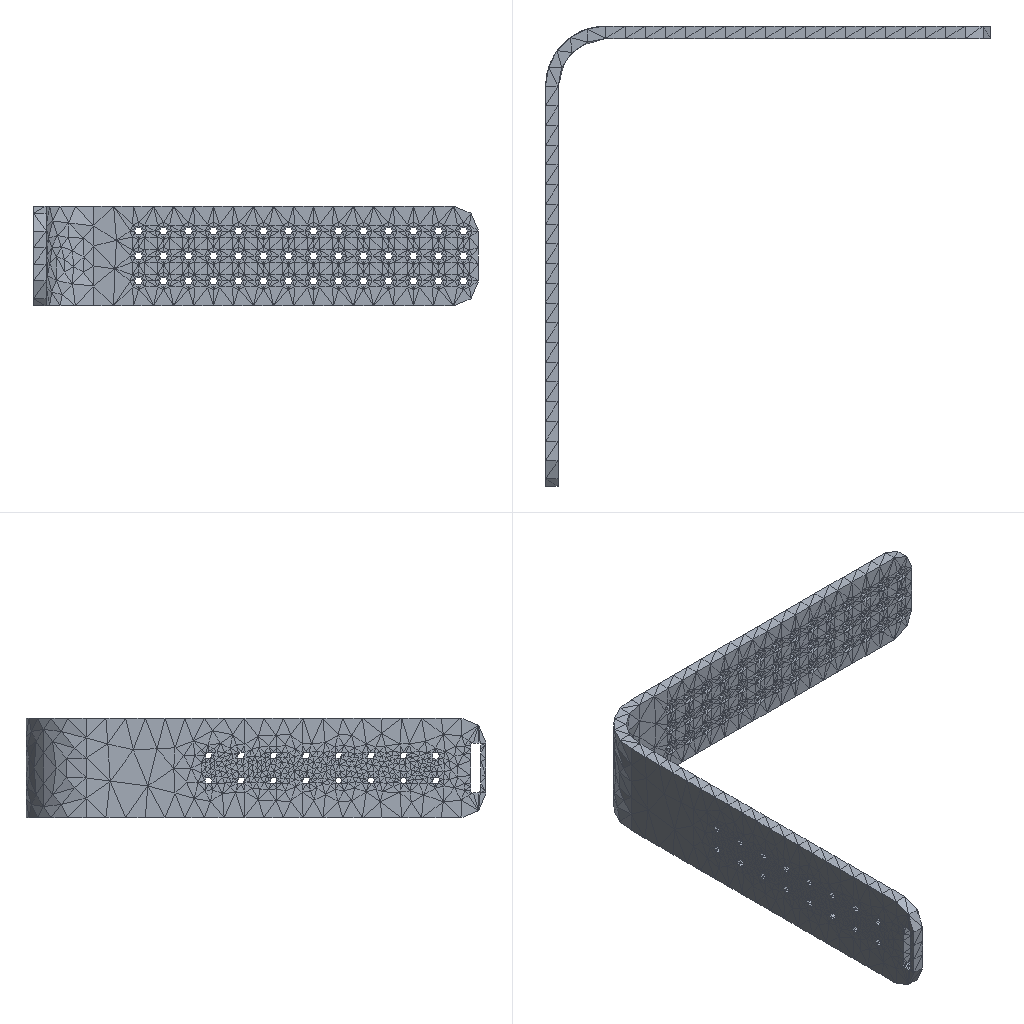Simulation study | ansys workbench
Set-up summary:
category,name,step,type,value,unit,region
solver,ansys_workbench
units,mm-N-s-tonne (MPa),,stated,"/units,MPA"
analysis,LS1,,static
load_step,LS1,LS1,static,nsubst=1; time=1
mesh,nodes,,,24678
mesh,elements,,,13329
element_type,SOLID187,,,13233
element_type,SURF154,,,96
material,Structural Steel,,E,200000,tonne s^-2 mm^-1
material,Structural Steel,,nu,0.3
material,Structural Steel,,density,7.85e-09,tonne mm^-3
material,Structural Steel,,conductivity,60.5,tonne mm s^-3 C^-1
material,Structural Steel,,specific_heat,4.34e+08,mm^2 s^-2 C^-1
material,Structural Steel,,cte,1.2e-05,C^-1
material,Structural Steel,,permeability,10000
material,Structural Steel,,resistivity,0.00017,ohm mm
load,Define Force Using Surface Effect Elements,LS1,surface-effect pres face 3,-0.06181,,SURF154 #2
bc,Fixed Supports,model,fixed,[dofs=ALL],,_FIXEDSU
named_set,_FIXEDSU,,node,192
Ansys APDL input file, long lists of numbers shortened:
/batch
/config,noeldb,1     ! force off writing results to database
*get,_wallstrt,active,,time,wall
! ANSYS input file written by Workbench version 2023 R1
/config,resuprec,0   ! write the result values in double precision for topology optimization future intent
! File used for geometry attach:
/title,daizuo41--____ (B5)
! ****** Begin Custom Load Command Snippet ******
/COM, ACT Extensions:
/COM,     LSDYNA, 2023.1
/COM,/COM,     ANSYSMotion, 2023.1
/COM,
! ****** End   Custom Load Command Snippet ******
*DIM,_wb_ProjectScratch_dir,string,248
_wb_ProjectScratch_dir(1) = ''
*DIM,_wb_SolverFiles_dir,string,248
_wb_SolverFiles_dir(1) = ''
*DIM,_wb_userfiles_dir,string,248
_wb_userfiles_dir(1) = ''
/com,--- Data in consistent NMM units. See Solving Units in the help system for more information.
/units,MPA
/nopr
/wb,file,start              !  signify a WB generated input file
/prep7
! Turn off shape checking because checks already performed inside WB mesher.
! See help system for more information.
SHPP,OFF,,NOWARN
/nolist
etcon,set             ! allow ANSYS to choose best KEYOP's for 180x elements, resets any applicable keyopt to MAPDL defaults
/com,*********** Nodes for the whole assembly ***********
nblock,3,,27145
(1i9,3e20.9e3)
        1     1.661341912E+02     1.790341912E+02     3.000000000E+01
! (24677 more lines like these left out)
-1
/wb,elem,start            !  set before creation of elements
/com,*********** Elements for Body 1 "plate1" ***********
et,1,187
eblock,19,solid,,13233
(19i9)
        1        1        1        1        0        0        0        0       10        0        1      465     4004      473     3975     7550     7607     7542     7549
! (26465 more lines like these left out)
-1
/wb,elem,end               !  done creating elements
/com,*********** Send User Defined Coordinate System(s) ***********
csys,0
toffst,273.15,  ! Temperature offset from absolute zero
/com,*********** Set Reference Temperature ***********
tref,22.
/wb,mat,start              !  starting to send materials
/com,*********** Send Materials ***********
Temperature = 'TEMP' ! Temperature
MP,DENS,1,7.85e-09,	! tonne mm^-3
MP,ALPX,1,1.2e-05,	! C^-1
MP,C,1,434000000,	! mm^2 s^-2 C^-1
MP,KXX,1,60.5,	! tonne mm s^-3 C^-1
MP,RSVX,1,0.00017,	! ohm mm
MP,EX,1,200000,	! tonne s^-2 mm^-1
MP,NUXY,1,0.3,
MP,MURX,1,10000,
/wb,mat,end                !  done sending materials
!************************* Model Summary ********************
!plate1,	结构钢,	matid,	1
!************************* End Model Summary ********************
! get the diagonal of the bounding box. Needed later for other things
*get,_xmin,node,,mnloc,x
*get,_ymin,node,,mnloc,y
*get,_zmin,node,,mnloc,z
*get,_xmax,node,,mxloc,x
*get,_ymax,node,,mxloc,y
*get,_zmax,node,,mxloc,z
_ASMDIAG=(_xmax-_xmin)*(_xmax-_xmin)+(_ymax-_ymin)*(_ymax-_ymin)+(_zmax-_zmin)*(_zmax-_zmin)
_ASMDIAG=SQRT(_ASMDIAG)
/wb,contact,start          !  starting to send contact
/wb,contact,end            !  done creating contacts
/golist
/wb,load,start             !  starting to send loads
/com,*********** Fixed Supports ***********
CMBLOCK,_FIXEDSU,NODE,      192
(8i10)
      1361      1362      1363      1364      1365      1366      1367      1368
! (23 more lines like these left out)
cmsel,s,_FIXEDSU
d,all,all
nsel,all
/com,*********** Define Force Using Surface Effect Elements ***********
local,12,0,0.,0.,0.,0.,0.,0.
csys,0
et,2,154
mat,2
eblock,10,,,96
(15i9)
    19988        2        2        2       12      789      786     3186     3186     9756     9760     3186     9776
! (95 more lines like these left out)
-1
esel,s,type,,2
keyop,2,2,1                ! Apply load in local coordinate system
keyop,2,7,1                ! Use original area so load is constant in large deformation
esel,all
/gst,on,on
fini
*get,_numnode,node,0,count
*get,_numelem,elem,0,count
*get, _MAXELEMNUM, elem, 0, NUM, MAX
*get, _MAXNODENUM, node, 0, NUM, MAX
*get, _MAXELEMTYPE, etyp, 0, NUM, MAX
*get, _MAXREALCONST, rcon, 0, NUM, MAX
/go
/wb,load,end               !  done creating loads
/com,--- Number of total nodes = %_numnode%
/com,--- Number of contact elements = 96
/com,--- Number of spring elements = 0
/com,--- Number of bearing elements = 0
/com,--- Number of solid elements = 13233
/com,--- Number of condensed parts = 0
/com,--- Number of total elements = %_numelem%
*get,_wallbsol,active,,time,wall
/com,****************************************************************************
/com,*************************    SOLUTION       ********************************
/com,****************************************************************************
/solu
antype,0                   ! static analysis
_thickRatio=  0     ! Ratio of thick parts in the model
eqsl,sparse,,,,,1
cntr,print,1               ! print out contact info and also make no initial contact an error
nldiag,cont,iter           ! print out contact info each equilibrium iteration
rescontrol,,none                 ! Do not keep any restart files
/com,****************************************************
/com,******************* SOLVE FOR LS 1 OF 1 ****************
esel,s,type,,2
nsle
sfe,all,1,pres,1,0.
sfe,all,2,pres,1,0.
sfe,all,3,pres,1,-6.18108500961187e-002
nsel,all
esel,all
/nopr
/gopr
nsub,1,1,1
time,1.
outres,erase
outres,all,none
outres,nsol,all  ! Output nodal forces at all time points for Topology Optimization future intent
outres,rsol,all
outres,eangl,all
outres,etmp,all
outres,veng,all
outres,nload,all  ! Output nodal forces at all time points for Topology Optimization future intent
outres,strs,all
outres,srfs,all
outres,bkstr,all
outres,epel,all,
outres,eppl,all,
outres,cont,all,
save, file_Static24, db ! Topology optimization database
! *********** WB SOLVE COMMAND ***********
! check interactive state
*get,ANSINTER_,active,,int
*if,ANSINTER_,ne,0,then
/eof
*endif
solve
/com *************** Write FE CONNECTORS *********
CEWRITE,file,ce,,INTE
/com,****************************************************
/com,*************** FINISHED SOLVE FOR LS 1 *************
*get,_wallasol,active,,time,wall
/nopr
*get,_numnode,node,0,count
*get,_numelem,elem,0,count
*get, _MAXELEMNUM, elem, 0, NUM, MAX
*get, _MAXNODENUM, node, 0, NUM, MAX,,,INTERNAL
*get, _MAXELEMTYPE, etyp, 0, NUM, MAX
*get, _MAXREALCONST, rcon, 0, NUM, MAX
*get,_NSOLTHREADS,active,0,ntfs
*get,_NSOLPROCESSES,active,0,npfs
/gopr
/post1
xmlo,ENCODING,ISO-8859-1
xmlo,parm
/xml,parm,xml
fini
/gopr
*get,_walldone,active,,time,wall
_preptime=(_wallbsol-_wallstrt)*3600
_solvtime=(_wallasol-_wallbsol)*3600
_posttime=(_walldone-_wallasol)*3600
_totaltim=(_walldone-_wallstrt)*3600
*get,_dlbratio,active,0,solu,dlbr
*get,_combtime,active,0,solu,comb
*get,_ssmode,active,0,solu,ssmm
*get,_ndofs,active,0,solu,ndof
/com,--- Total number of nodes = %_numnode%
/com,--- Total number of elements = %_numelem%
/com,--- Element load balance ratio = %_dlbratio%
/com,--- Time to combine distributed files = %_combtime%
/com,--- Sparse memory mode = %_ssmode%
/com,--- Number of DOF = %_ndofs%
/wb,file,end               ! done with WB generated input
Results summary:
result,analyses[0].index,,,1
result,analyses[0].system,,,SYS
result,analyses[0].deck,,,deck.dat
result,analyses[0].solve_status,,,completed
result,analyses[0].analysis_type,,,static
result,analyses[0].physics,,,mechanical
result,analyses[0].unit_system,,,"NMM: mm, ton, N, s, mV, mA, degC"
result,analyses[0].n_sets,,,1
result,analyses[0].load_steps[0].set,set=1,,1
result,analyses[0].load_steps[0].time_or_freq,set=1,,1
result,analyses[0].load_steps[0].max_displacement_magnitude,set=1,,0.2124
result,analyses[0].load_steps[0].max_von_mises_nodal,set=1,,17.175
result,analyses[0].load_steps[0].reaction_force_sum_xyz[1],set=1,,-3.2278e-08
result,analyses[0].load_steps[0].reaction_force_sum_xyz[2],set=1,,1.49689e-08
result,analyses[0].load_steps[0].reaction_force_sum_xyz[3],set=1,,11.995
result,geometry_export[0][0],,,.step
result,geometry_export[0][1],,,ok
result,geometry_export[0][2],,,1